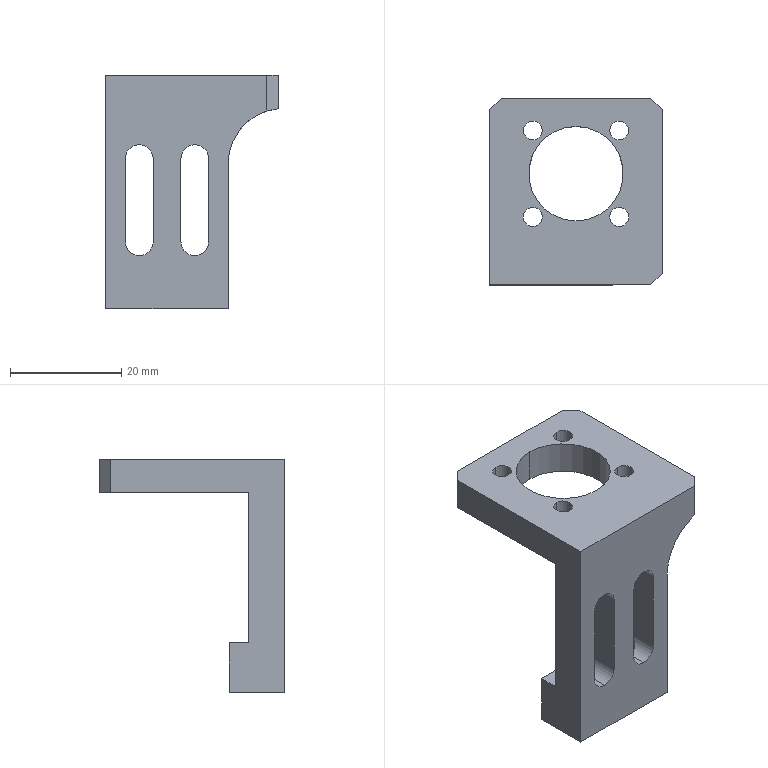NC program | NX | posted with a generic post | part box 31 x 33.478 x 42 mm
Lines 3048 to 3423 of 3423:
(ZLEVEL_PROFILE_1 , TOOL : D10JING)
N6076 T14 M6
N6078 G54
N6080 G17 G0 G90 X-22.309 Y-18.361 B0. C0. S9500 M3
N6082 G43 Z30. H14
N6084 Z-12.5
N6086 G94 G1 Z-14. F1000.
N6088 X-21. Y-17.605
N6090 G3 X-20.5 Y-16.739 R1.
N6092 G1 Y14.739 F1500.
N6094 G2 X-19.036 Y18.275 R5.
N6096 G1 X-17.036 Y20.275
N6098 G2 X-13.5 Y21.739 R5.
N6100 G1 X13.5
N6102 G2 X17.036 Y20.275 R5.
N6104 G1 X19.036 Y18.275
N6106 G2 X20.5 Y14.739 R5.
N6108 G1 Y-14.739
N6110 G2 X19.036 Y-18.275 R5.
N6112 G1 X17.036 Y-20.275
N6114 G2 X13.5 Y-21.739 R5.
N6116 G1 X-15.5
N6118 G2 X-20.5 Y-16.739 R5.
N6120 G1 Y14.739 Z-16.81
N6122 X-20.492 Y15.019 Z-16.835
N6124 X-20.469 Y15.299 Z-16.86
N6126 X-20.429 Y15.577 Z-16.885
N6128 X-20.375 Y15.852 Z-16.91
N6130 X-20.305 Y16.123 Z-16.935
N6132 X-20.219 Y16.39 Z-16.96
N6134 X-20.119 Y16.653 Z-16.985
N6136 X-20.005 Y16.909 Z-17.01
N6138 X-19.876 Y17.158 Z-17.035
N6140 X-19.734 Y17.399 Z-17.06
N6142 X-19.578 Y17.632 Z-17.085
N6144 X-19.409 Y17.857 Z-17.11
N6146 X-19.228 Y18.071 Z-17.135
N6148 X-19.036 Y18.275 Z-17.16
N6150 X-17.036 Y20.275 Z-17.413
N6152 X-16.832 Y20.467 Z-17.438
N6154 X-16.617 Y20.648 Z-17.463
N6156 X-16.393 Y20.817 Z-17.488
N6158 X-16.16 Y20.973 Z-17.513
N6160 X-15.919 Y21.115 Z-17.538
N6162 X-15.669 Y21.244 Z-17.563
N6164 X-15.413 Y21.358 Z-17.588
N6166 X-15.151 Y21.459 Z-17.613
N6168 X-14.884 Y21.544 Z-17.638
N6170 X-14.613 Y21.614 Z-17.663
N6172 X-14.338 Y21.668 Z-17.688
N6174 X-14.06 Y21.708 Z-17.713
N6176 X-13.78 Y21.731 Z-17.738
N6178 X-13.5 Y21.739 Z-17.763
N6180 X13.5 Z-20.173
N6182 X13.78 Y21.731 Z-20.198
N6184 X14.06 Y21.708 Z-20.223
N6186 X14.338 Y21.668 Z-20.248
N6188 X14.613 Y21.614 Z-20.273
N6190 X14.884 Y21.544 Z-20.298
N6192 X15.151 Y21.459 Z-20.323
N6194 X15.413 Y21.358 Z-20.348
N6196 X15.669 Y21.244 Z-20.373
N6198 X15.919 Y21.115 Z-20.398
N6200 X16.16 Y20.973 Z-20.423
N6202 X16.393 Y20.817 Z-20.448
N6204 X16.617 Y20.648 Z-20.473
N6206 X16.832 Y20.467 Z-20.498
N6208 X17.036 Y20.275 Z-20.523
N6210 X19.036 Y18.275 Z-20.776
N6212 X19.228 Y18.071 Z-20.801
N6214 X19.409 Y17.857 Z-20.826
N6216 X19.578 Y17.632 Z-20.851
N6218 X19.734 Y17.399 Z-20.876
N6220 X19.876 Y17.158 Z-20.901
N6222 X20.005 Y16.909 Z-20.926
N6224 X20.119 Y16.653 Z-20.951
N6226 X20.219 Y16.39 Z-20.976
N6228 X20.305 Y16.123 Z-21.001
N6230 X20.375 Y15.852 Z-21.026
N6232 X20.429 Y15.577 Z-21.051
N6234 X20.469 Y15.299 Z-21.076
N6236 X20.492 Y15.019 Z-21.101
N6238 X20.5 Y14.739 Z-21.126
N6240 Y-14.739 Z-23.758
N6242 X20.492 Y-15.019 Z-23.783
N6244 X20.469 Y-15.299 Z-23.808
N6246 X20.429 Y-15.577 Z-23.833
N6248 X20.375 Y-15.852 Z-23.858
N6250 X20.305 Y-16.123 Z-23.883
N6252 X20.219 Y-16.39 Z-23.908
N6254 X20.119 Y-16.653 Z-23.933
N6256 X20.005 Y-16.909 Z-23.958
N6258 X19.876 Y-17.158 Z-23.983
N6260 X19.734 Y-17.399 Z-24.008
N6262 X19.578 Y-17.632 Z-24.033
N6264 X19.409 Y-17.857 Z-24.058
N6266 X19.228 Y-18.071 Z-24.083
N6268 X19.036 Y-18.275 Z-24.108
N6270 X17.036 Y-20.275 Z-24.36
N6272 X16.832 Y-20.467 Z-24.385
N6274 X16.617 Y-20.648 Z-24.41
N6276 X16.393 Y-20.817 Z-24.435
N6278 X16.16 Y-20.973 Z-24.46
N6280 X15.919 Y-21.115 Z-24.486
N6282 X15.669 Y-21.244 Z-24.511
N6284 X15.413 Y-21.358 Z-24.536
N6286 X15.151 Y-21.459 Z-24.561
N6288 X14.884 Y-21.544 Z-24.586
N6290 X14.613 Y-21.614 Z-24.611
N6292 X14.338 Y-21.668 Z-24.636
N6294 X14.06 Y-21.708 Z-24.661
N6296 X13.78 Y-21.731 Z-24.686
N6298 X13.5 Y-21.739 Z-24.711
N6300 X-15.5 Z-27.299
N6302 X-15.802 Y-21.73 Z-27.326
N6304 X-16.103 Y-21.703 Z-27.353
N6306 X-16.401 Y-21.657 Z-27.38
N6308 X-16.697 Y-21.594 Z-27.407
N6310 X-16.988 Y-21.513 Z-27.434
N6312 X-17.273 Y-21.414 Z-27.461
N6314 X-17.552 Y-21.299 Z-27.488
N6316 X-17.824 Y-21.166 Z-27.515
N6318 X-18.087 Y-21.018 Z-27.542
N6320 X-18.34 Y-20.854 Z-27.569
N6322 X-18.584 Y-20.675 Z-27.596
N6324 X-18.816 Y-20.482 Z-27.623
N6326 X-19.036 Y-20.275 Z-27.65
N6328 X-19.243 Y-20.055 Z-27.677
N6330 X-19.436 Y-19.823 Z-27.704
N6332 X-19.615 Y-19.579 Z-27.731
N6334 X-19.779 Y-19.326 Z-27.757
N6336 X-19.927 Y-19.063 Z-27.784
N6338 X-20.06 Y-18.791 Z-27.811
N6340 X-20.175 Y-18.512 Z-27.838
N6342 X-20.274 Y-18.227 Z-27.865
N6344 X-20.355 Y-17.936 Z-27.892
N6346 X-20.418 Y-17.64 Z-27.919
N6348 X-20.464 Y-17.342 Z-27.946
N6350 X-20.491 Y-17.041 Z-27.973
N6352 X-20.5 Y-16.739 Z-28.
N6354 Y14.739 Z-30.81
N6356 X-20.492 Y15.019 Z-30.835
N6358 X-20.469 Y15.299 Z-30.86
N6360 X-20.429 Y15.577 Z-30.885
N6362 X-20.375 Y15.852 Z-30.91
N6364 X-20.305 Y16.123 Z-30.935
N6366 X-20.219 Y16.39 Z-30.96
N6368 X-20.119 Y16.653 Z-30.985
N6370 X-20.005 Y16.909 Z-31.01
N6372 X-19.876 Y17.158 Z-31.035
N6374 X-19.734 Y17.399 Z-31.06
N6376 X-19.578 Y17.632 Z-31.085
N6378 X-19.409 Y17.857 Z-31.11
N6380 X-19.228 Y18.071 Z-31.135
N6382 X-19.036 Y18.275 Z-31.16
N6384 X-17.036 Y20.275 Z-31.413
N6386 X-16.832 Y20.467 Z-31.438
N6388 X-16.617 Y20.648 Z-31.463
N6390 X-16.393 Y20.817 Z-31.488
N6392 X-16.16 Y20.973 Z-31.513
N6394 X-15.919 Y21.115 Z-31.538
N6396 X-15.669 Y21.244 Z-31.563
N6398 X-15.413 Y21.358 Z-31.588
N6400 X-15.151 Y21.459 Z-31.613
N6402 X-14.884 Y21.544 Z-31.638
N6404 X-14.613 Y21.614 Z-31.663
N6406 X-14.338 Y21.668 Z-31.688
N6408 X-14.06 Y21.708 Z-31.713
N6410 X-13.78 Y21.731 Z-31.738
N6412 X-13.5 Y21.739 Z-31.763
N6414 X13.5 Z-34.173
N6416 X13.78 Y21.731 Z-34.198
N6418 X14.06 Y21.708 Z-34.223
N6420 X14.338 Y21.668 Z-34.248
N6422 X14.613 Y21.614 Z-34.273
N6424 X14.884 Y21.544 Z-34.298
N6426 X15.151 Y21.459 Z-34.323
N6428 X15.413 Y21.358 Z-34.348
N6430 X15.669 Y21.244 Z-34.373
N6432 X15.919 Y21.115 Z-34.398
N6434 X16.16 Y20.973 Z-34.423
N6436 X16.393 Y20.817 Z-34.448
N6438 X16.617 Y20.648 Z-34.473
N6440 X16.832 Y20.467 Z-34.498
N6442 X17.036 Y20.275 Z-34.523
N6444 X19.036 Y18.275 Z-34.776
N6446 X19.228 Y18.071 Z-34.801
N6448 X19.409 Y17.857 Z-34.826
N6450 X19.578 Y17.632 Z-34.851
N6452 X19.734 Y17.399 Z-34.876
N6454 X19.876 Y17.158 Z-34.901
N6456 X20.005 Y16.909 Z-34.926
N6458 X20.119 Y16.653 Z-34.951
N6460 X20.219 Y16.39 Z-34.976
N6462 X20.305 Y16.123 Z-35.001
N6464 X20.375 Y15.852 Z-35.026
N6466 X20.429 Y15.577 Z-35.051
N6468 X20.469 Y15.299 Z-35.076
N6470 X20.492 Y15.019 Z-35.101
N6472 X20.5 Y14.739 Z-35.126
N6474 Y-14.739 Z-37.758
N6476 X20.492 Y-15.019 Z-37.783
N6478 X20.469 Y-15.299 Z-37.808
N6480 X20.429 Y-15.577 Z-37.833
N6482 X20.375 Y-15.852 Z-37.858
N6484 X20.305 Y-16.123 Z-37.883
N6486 X20.219 Y-16.39 Z-37.908
N6488 X20.119 Y-16.653 Z-37.933
N6490 X20.005 Y-16.909 Z-37.958
N6492 X19.876 Y-17.158 Z-37.983
N6494 X19.734 Y-17.399 Z-38.008
N6496 X19.578 Y-17.632 Z-38.033
N6498 X19.409 Y-17.857 Z-38.058
N6500 X19.228 Y-18.071 Z-38.083
N6502 X19.036 Y-18.275 Z-38.108
N6504 X17.036 Y-20.275 Z-38.36
N6506 X16.832 Y-20.467 Z-38.385
N6508 X16.617 Y-20.648 Z-38.41
N6510 X16.393 Y-20.817 Z-38.435
N6512 X16.16 Y-20.973 Z-38.46
N6514 X15.919 Y-21.115 Z-38.486
N6516 X15.669 Y-21.244 Z-38.511
N6518 X15.413 Y-21.358 Z-38.536
N6520 X15.151 Y-21.459 Z-38.561
N6522 X14.884 Y-21.544 Z-38.586
N6524 X14.613 Y-21.614 Z-38.611
N6526 X14.338 Y-21.668 Z-38.636
N6528 X14.06 Y-21.708 Z-38.661
N6530 X13.78 Y-21.731 Z-38.686
N6532 X13.5 Y-21.739 Z-38.711
N6534 X-15.5 Z-41.299
N6536 X-15.802 Y-21.73 Z-41.326
N6538 X-16.103 Y-21.703 Z-41.353
N6540 X-16.401 Y-21.657 Z-41.38
N6542 X-16.697 Y-21.594 Z-41.407
N6544 X-16.988 Y-21.513 Z-41.434
N6546 X-17.273 Y-21.414 Z-41.461
N6548 X-17.552 Y-21.299 Z-41.488
N6550 X-17.824 Y-21.166 Z-41.515
N6552 X-18.087 Y-21.018 Z-41.542
N6554 X-18.34 Y-20.854 Z-41.569
N6556 X-18.584 Y-20.675 Z-41.596
N6558 X-18.816 Y-20.482 Z-41.623
N6560 X-19.036 Y-20.275 Z-41.65
N6562 X-19.243 Y-20.055 Z-41.677
N6564 X-19.436 Y-19.823 Z-41.704
N6566 X-19.615 Y-19.579 Z-41.731
N6568 X-19.779 Y-19.326 Z-41.757
N6570 X-19.927 Y-19.063 Z-41.784
N6572 X-20.06 Y-18.791 Z-41.811
N6574 X-20.175 Y-18.512 Z-41.838
N6576 X-20.274 Y-18.227 Z-41.865
N6578 X-20.355 Y-17.936 Z-41.892
N6580 X-20.418 Y-17.64 Z-41.919
N6582 X-20.464 Y-17.342 Z-41.946
N6584 X-20.491 Y-17.041 Z-41.973
N6586 X-20.5 Y-16.739 Z-42.
N6588 Y14.739
N6590 G2 X-19.036 Y18.275 R5.
N6592 G1 X-17.036 Y20.275
N6594 G2 X-13.5 Y21.739 R5.
N6596 G1 X13.5
N6598 G2 X17.036 Y20.275 R5.
N6600 G1 X19.036 Y18.275
N6602 G2 X20.5 Y14.739 R5.
N6604 G1 Y-14.739
N6606 G2 X19.036 Y-18.275 R5.
N6608 G1 X17.036 Y-20.275
N6610 G2 X13.5 Y-21.739 R5.
N6612 G1 X-15.5
N6614 G2 X-20.5 Y-16.739 R5.
N6616 G3 X-21. Y-15.873 R1.
N6618 G1 X-22.5 Y-15.007
N6620 Z-40.5
N6622 G0 Z30.
(HOLE_MILLING , TOOL : D10JING)
N6624 X0. Y3.261
N6626 Z0.5
N6628 G3 X1.75 Y1.511 R1.75
N6630 X3.5 Y3.261 R1.75
N6632 X3.5 Y3.261 Z-0.1 I-3.5 J0.
N6634 X3.5 Y3.261 Z-0.7 I-3.5 J0.
N6636 X3.5 Y3.261 Z-1.3 I-3.5 J0.
N6638 X3.5 Y3.261 Z-1.9 I-3.5 J0.
N6640 X3.5 Y3.261 Z-2.5 I-3.5 J0.
N6642 X3.5 Y3.261 Z-3.1 I-3.5 J0.
N6644 X3.5 Y3.261 Z-3.7 I-3.5 J0.
N6646 X3.5 Y3.261 Z-4.3 I-3.5 J0.
N6648 X3.5 Y3.261 Z-4.9 I-3.5 J0.
N6650 X3.5 Y3.261 Z-5.5 I-3.5 J0.
N6652 X1.75 Y0.23 Z-6. R-3.5
N6654 X3.031 Y5.011 R3.5
N6656 X1.75 Y0.23 R-3.5
N6658 X2.391 Y2.62 R1.75
N6660 X0. Y3.261 R1.75
N6662 G0 Z30.
N6664 M5
(PLANAR_MILL_COPY , TOOL : D6A45)
N6666 T01 M6
N6668 G54
N6670 G17 G0 G90 X8.328 Y-4.95 B0. C0. S9500 M3
N6672 G43 Z30. H1
N6674 Z0.5
N6676 G94 G1 Z-1. F1250.
N6678 G3 X8.578 Y-4.517 R0.5
N6680 X7.778 Y-3.717 R0.8
N6682 X8.578 Y-4.517 R-0.8
N6684 X8.328 Y-4.084 R0.5
N6686 G1 Z0.5
N6688 G0 Z30.
N6690 X16.9 Y0.866
N6692 Z0.5
N6694 G1 Z-1.
N6696 G3 X16.4 Y0. R1.
N6698 G1 Y-14.739
N6700 G2 X16.136 Y-15.375 R0.9
N6702 G1 X14.136 Y-17.375
N6704 G2 X13.5 Y-17.639 R0.9
N6706 G1 X-15.5
N6708 G2 X-16.4 Y-16.739 R0.9
N6710 G1 Y14.739
N6712 G2 X-16.136 Y15.375 R0.9
N6714 G1 X-14.136 Y17.375
N6716 G2 X-13.5 Y17.639 R0.9
N6718 G1 X13.5
N6720 G2 X14.136 Y17.375 R0.9
N6722 G1 X16.136 Y15.375
N6724 G2 X16.4 Y14.739 R0.9
N6726 G1 Y0.
N6728 G3 X16.9 Y-0.866 R1.
N6730 G1 Z0.5
N6732 G0 Z30.
N6734 X-8.328 Y-4.084
N6736 Z0.5
N6738 G1 Z-1.
N6740 G3 X-8.578 Y-4.517 R0.5
N6742 X-7.778 Y-5.317 R0.8
N6744 X-8.578 Y-4.517 R-0.8
N6746 X-8.328 Y-4.95 R0.5
N6748 G1 Z0.5
N6750 G0 Z30.
N6752 X-7.1 Y4.127
N6754 Z0.5
N6756 G1 Z-1.
N6758 G3 X-7.6 Y3.261 R1.
N6760 X0. Y-4.339 R7.6
N6762 X-7.6 Y3.261 R-7.6
N6764 X-7.1 Y2.395 R1.
N6766 G1 Z0.5
N6768 G0 Z30.
N6770 X-7.345 Y11.589
N6772 Z0.5
N6774 G1 Z-1.
N6776 G3 X-7.778 Y11.839 R0.5
N6778 X-8.578 Y11.039 R0.8
N6780 X-7.778 Y11.839 R-0.8
N6782 X-8.211 Y11.589 R0.5
N6784 G1 Z0.5
N6786 G0 Z30.
N6788 X8.211
N6790 Z0.5
N6792 G1 Z-1.
N6794 G3 X7.778 Y11.839 R0.5
N6796 X6.978 Y11.039 R0.8
N6798 X7.778 Y11.839 R-0.8
N6800 X7.345 Y11.589 R0.5
N6802 G1 Z0.5
N6804 G0 Z30.
N6806 M5
N6808 M2